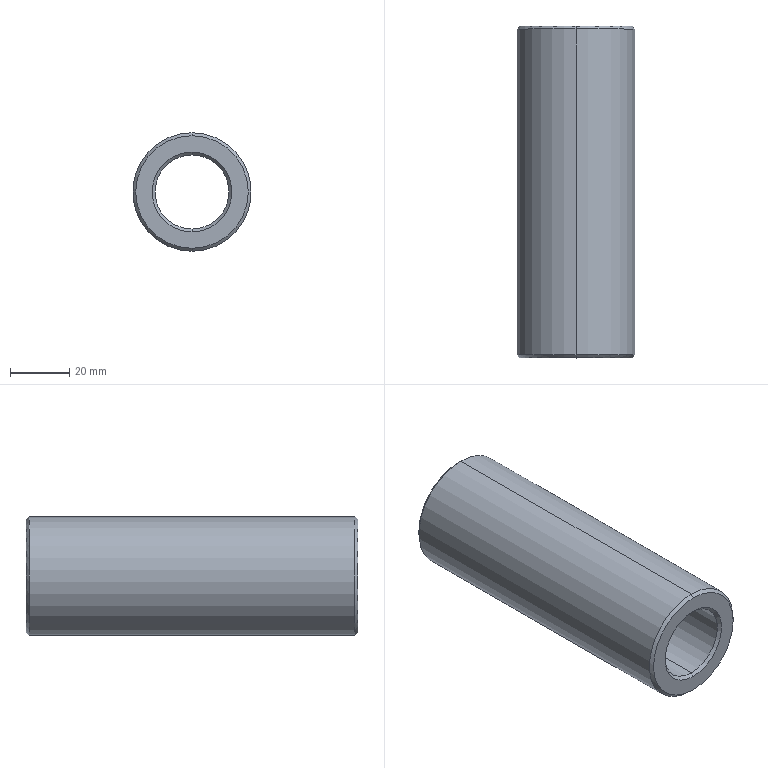Part | SolidWorks | features Chamfer 1, Extrusion 1 | 1 solid | 14 faces | box 40 x 112 x 40 mm | volume 85561 mm3 | cone 8 | cylinder 4 | plane 2 | commonest cylinder face diameters 25 x2 40 x2
STEP:
#1=CARTESIAN_POINT('',(0.,111.,-12.5));
#2=VERTEX_POINT('',#1);
#3=CARTESIAN_POINT('',(0.,111.,12.5));
#4=VERTEX_POINT('',#3);
#5=CARTESIAN_POINT('',(0.,111.,0.));
#6=DIRECTION('',(0.,1.,0.));
#7=DIRECTION('',(0.,0.,1.));
#8=AXIS2_PLACEMENT_3D('',#5,#6,#7);
#9=CIRCLE('',#8,12.5);
#10=EDGE_CURVE('',#2,#4,#9,.T.);
#11=ORIENTED_EDGE('',*,*,#10,.F.);
#12=CARTESIAN_POINT('',(0.,112.,-13.5));
#13=VERTEX_POINT('',#12);
#14=CARTESIAN_POINT('',(0.,111.,-12.5));
#15=DIRECTION('',(0.,0.7071,-0.7071));
#16=VECTOR('',#15,1000.);
#17=LINE('',#14,#16);
#18=EDGE_CURVE('',#2,#13,#17,.T.);
#19=ORIENTED_EDGE('',*,*,#18,.T.);
#20=CARTESIAN_POINT('',(0.,112.,13.5));
#21=VERTEX_POINT('',#20);
#22=CARTESIAN_POINT('',(0.,112.,0.));
#23=DIRECTION('',(0.,-1.,0.));
#24=DIRECTION('',(0.,0.,1.));
#25=AXIS2_PLACEMENT_3D('',#22,#23,#24);
#26=CIRCLE('',#25,13.5);
#27=EDGE_CURVE('',#21,#13,#26,.T.);
#28=ORIENTED_EDGE('',*,*,#27,.F.);
#29=CARTESIAN_POINT('',(0.,111.,12.5));
#30=DIRECTION('',(0.,0.7071,0.7071));
#31=VECTOR('',#30,1000.);
#32=LINE('',#29,#31);
#33=EDGE_CURVE('',#4,#21,#32,.T.);
#34=ORIENTED_EDGE('',*,*,#33,.F.);
#35=EDGE_LOOP('',(#11,#19,#28,#34));
#36=FACE_OUTER_BOUND('',#35,.T.);
#37=CARTESIAN_POINT('',(0.,111.,0.));
#38=DIRECTION('',(0.,1.,0.));
#39=DIRECTION('',(0.,0.,1.));
#40=AXIS2_PLACEMENT_3D('',#37,#38,#39);
#41=CONICAL_SURFACE('',#40,12.5,0.7854);
#42=ADVANCED_FACE('',(#36),#41,.F.);
#43=CARTESIAN_POINT('',(0.,1.,12.5));
#44=VERTEX_POINT('',#43);
#45=CARTESIAN_POINT('',(0.,1.,-12.5));
#46=VERTEX_POINT('',#45);
#47=CARTESIAN_POINT('',(0.,1.,0.));
#48=DIRECTION('',(0.,-1.,0.));
#49=DIRECTION('',(0.,0.,1.));
#50=AXIS2_PLACEMENT_3D('',#47,#48,#49);
#51=CIRCLE('',#50,12.5);
#52=EDGE_CURVE('',#44,#46,#51,.T.);
#53=ORIENTED_EDGE('',*,*,#52,.F.);
#54=CARTESIAN_POINT('',(0.,0.,13.5));
#55=VERTEX_POINT('',#54);
#56=CARTESIAN_POINT('',(0.,0.,13.5));
#57=DIRECTION('',(0.,-0.7071,0.7071));
#58=VECTOR('',#57,1000.);
#59=LINE('',#56,#58);
#60=EDGE_CURVE('',#44,#55,#59,.T.);
#61=ORIENTED_EDGE('',*,*,#60,.T.);
#62=CARTESIAN_POINT('',(0.,0.,-13.5));
#63=VERTEX_POINT('',#62);
#64=CARTESIAN_POINT('',(0.,0.,0.));
#65=DIRECTION('',(0.,1.,0.));
#66=DIRECTION('',(0.,0.,1.));
#67=AXIS2_PLACEMENT_3D('',#64,#65,#66);
#68=CIRCLE('',#67,13.5);
#69=EDGE_CURVE('',#63,#55,#68,.T.);
#70=ORIENTED_EDGE('',*,*,#69,.F.);
#71=CARTESIAN_POINT('',(0.,0.,-13.5));
#72=DIRECTION('',(0.,-0.7071,-0.7071));
#73=VECTOR('',#72,1000.);
#74=LINE('',#71,#73);
#75=EDGE_CURVE('',#46,#63,#74,.T.);
#76=ORIENTED_EDGE('',*,*,#75,.F.);
#77=EDGE_LOOP('',(#53,#61,#70,#76));
#78=FACE_OUTER_BOUND('',#77,.T.);
#79=CARTESIAN_POINT('',(0.,0.,0.));
#80=DIRECTION('',(0.,-1.,0.));
#81=DIRECTION('',(0.,0.,-1.));
#82=AXIS2_PLACEMENT_3D('',#79,#80,#81);
#83=CONICAL_SURFACE('',#82,13.5,0.7854);
#84=ADVANCED_FACE('',(#78),#83,.F.);
#85=CARTESIAN_POINT('',(0.,112.,19.));
#86=VERTEX_POINT('',#85);
#87=CARTESIAN_POINT('',(0.,112.,-19.));
#88=VERTEX_POINT('',#87);
#89=CARTESIAN_POINT('',(0.,112.,0.));
#90=DIRECTION('',(0.,1.,0.));
#91=DIRECTION('',(0.,0.,1.));
#92=AXIS2_PLACEMENT_3D('',#89,#90,#91);
#93=CIRCLE('',#92,19.);
#94=EDGE_CURVE('',#86,#88,#93,.T.);
#95=ORIENTED_EDGE('',*,*,#94,.F.);
#96=CARTESIAN_POINT('',(0.,111.,20.));
#97=VERTEX_POINT('',#96);
#98=CARTESIAN_POINT('',(0.,112.,19.));
#99=DIRECTION('',(0.,-0.7071,0.7071));
#100=VECTOR('',#99,1000.);
#101=LINE('',#98,#100);
#102=EDGE_CURVE('',#86,#97,#101,.T.);
#103=ORIENTED_EDGE('',*,*,#102,.T.);
#104=CARTESIAN_POINT('',(0.,111.,-20.));
#105=VERTEX_POINT('',#104);
#106=CARTESIAN_POINT('',(0.,111.,0.));
#107=DIRECTION('',(0.,-1.,0.));
#108=DIRECTION('',(0.,0.,1.));
#109=AXIS2_PLACEMENT_3D('',#106,#107,#108);
#110=CIRCLE('',#109,20.);
#111=EDGE_CURVE('',#105,#97,#110,.T.);
#112=ORIENTED_EDGE('',*,*,#111,.F.);
#113=CARTESIAN_POINT('',(0.,112.,-19.));
#114=DIRECTION('',(0.,-0.7071,-0.7071));
#115=VECTOR('',#114,1000.);
#116=LINE('',#113,#115);
#117=EDGE_CURVE('',#88,#105,#116,.T.);
#118=ORIENTED_EDGE('',*,*,#117,.F.);
#119=EDGE_LOOP('',(#95,#103,#112,#118));
#120=FACE_OUTER_BOUND('',#119,.T.);
#121=CARTESIAN_POINT('',(0.,112.,0.));
#122=DIRECTION('',(0.,-1.,0.));
#123=DIRECTION('',(0.,0.,-1.));
#124=AXIS2_PLACEMENT_3D('',#121,#122,#123);
#125=CONICAL_SURFACE('',#124,19.,0.7854);
#126=ADVANCED_FACE('',(#120),#125,.T.);
#127=CARTESIAN_POINT('',(0.,0.,-19.));
#128=VERTEX_POINT('',#127);
#129=CARTESIAN_POINT('',(0.,0.,19.));
#130=VERTEX_POINT('',#129);
#131=CARTESIAN_POINT('',(0.,0.,0.));
#132=DIRECTION('',(0.,-1.,0.));
#133=DIRECTION('',(0.,0.,1.));
#134=AXIS2_PLACEMENT_3D('',#131,#132,#133);
#135=CIRCLE('',#134,19.);
#136=EDGE_CURVE('',#128,#130,#135,.T.);
#137=ORIENTED_EDGE('',*,*,#136,.F.);
#138=CARTESIAN_POINT('',(0.,1.,-20.));
#139=VERTEX_POINT('',#138);
#140=CARTESIAN_POINT('',(0.,1.,-20.));
#141=DIRECTION('',(0.,0.7071,-0.7071));
#142=VECTOR('',#141,1000.);
#143=LINE('',#140,#142);
#144=EDGE_CURVE('',#128,#139,#143,.T.);
#145=ORIENTED_EDGE('',*,*,#144,.T.);
#146=CARTESIAN_POINT('',(0.,1.,20.));
#147=VERTEX_POINT('',#146);
#148=CARTESIAN_POINT('',(0.,1.,0.));
#149=DIRECTION('',(0.,1.,0.));
#150=DIRECTION('',(0.,0.,1.));
#151=AXIS2_PLACEMENT_3D('',#148,#149,#150);
#152=CIRCLE('',#151,20.);
#153=EDGE_CURVE('',#147,#139,#152,.T.);
#154=ORIENTED_EDGE('',*,*,#153,.F.);
#155=CARTESIAN_POINT('',(0.,1.,20.));
#156=DIRECTION('',(0.,0.7071,0.7071));
#157=VECTOR('',#156,1000.);
#158=LINE('',#155,#157);
#159=EDGE_CURVE('',#130,#147,#158,.T.);
#160=ORIENTED_EDGE('',*,*,#159,.F.);
#161=EDGE_LOOP('',(#137,#145,#154,#160));
#162=FACE_OUTER_BOUND('',#161,.T.);
#163=CARTESIAN_POINT('',(0.,1.,0.));
#164=DIRECTION('',(0.,1.,0.));
#165=DIRECTION('',(0.,0.,1.));
#166=AXIS2_PLACEMENT_3D('',#163,#164,#165);
#167=CONICAL_SURFACE('',#166,20.,0.7854);
#168=ADVANCED_FACE('',(#162),#167,.T.);
#169=ORIENTED_EDGE('',*,*,#10,.T.);
#170=CARTESIAN_POINT('',(0.,112.,12.5));
#171=DIRECTION('',(0.,-1.,0.));
#172=VECTOR('',#171,1000.);
#173=LINE('',#170,#172);
#174=EDGE_CURVE('',#4,#44,#173,.T.);
#175=ORIENTED_EDGE('',*,*,#174,.T.);
#176=ORIENTED_EDGE('',*,*,#52,.T.);
#177=CARTESIAN_POINT('',(0.,112.,-12.5));
#178=DIRECTION('',(0.,-1.,0.));
#179=VECTOR('',#178,1000.);
#180=LINE('',#177,#179);
#181=EDGE_CURVE('',#2,#46,#180,.T.);
#182=ORIENTED_EDGE('',*,*,#181,.F.);
#183=EDGE_LOOP('',(#169,#175,#176,#182));
#184=FACE_OUTER_BOUND('',#183,.T.);
#185=CARTESIAN_POINT('',(0.,112.,0.));
#186=DIRECTION('',(0.,-1.,0.));
#187=DIRECTION('',(0.,0.,-1.));
#188=AXIS2_PLACEMENT_3D('',#185,#186,#187);
#189=CYLINDRICAL_SURFACE('',#188,12.5);
#190=ADVANCED_FACE('',(#184),#189,.F.);
#191=ORIENTED_EDGE('',*,*,#111,.T.);
#192=CARTESIAN_POINT('',(0.,112.,20.));
#193=DIRECTION('',(0.,-1.,0.));
#194=VECTOR('',#193,1000.);
#195=LINE('',#192,#194);
#196=EDGE_CURVE('',#97,#147,#195,.T.);
#197=ORIENTED_EDGE('',*,*,#196,.T.);
#198=ORIENTED_EDGE('',*,*,#153,.T.);
#199=CARTESIAN_POINT('',(0.,112.,-20.));
#200=DIRECTION('',(0.,-1.,0.));
#201=VECTOR('',#200,1000.);
#202=LINE('',#199,#201);
#203=EDGE_CURVE('',#105,#139,#202,.T.);
#204=ORIENTED_EDGE('',*,*,#203,.F.);
#205=EDGE_LOOP('',(#191,#197,#198,#204));
#206=FACE_OUTER_BOUND('',#205,.T.);
#207=CARTESIAN_POINT('',(0.,112.,0.));
#208=DIRECTION('',(0.,-1.,0.));
#209=DIRECTION('',(0.,0.,-1.));
#210=AXIS2_PLACEMENT_3D('',#207,#208,#209);
#211=CYLINDRICAL_SURFACE('',#210,20.);
#212=ADVANCED_FACE('',(#206),#211,.T.);
#213=CARTESIAN_POINT('',(0.,112.,0.));
#214=DIRECTION('',(0.,1.,0.));
#215=DIRECTION('',(0.,0.,1.));
#216=AXIS2_PLACEMENT_3D('',#213,#214,#215);
#217=CIRCLE('',#216,19.);
#218=EDGE_CURVE('',#88,#86,#217,.T.);
#219=ORIENTED_EDGE('',*,*,#218,.T.);
#220=ORIENTED_EDGE('',*,*,#94,.T.);
#221=EDGE_LOOP('',(#219,#220));
#222=FACE_OUTER_BOUND('',#221,.T.);
#223=ORIENTED_EDGE('',*,*,#27,.T.);
#224=CARTESIAN_POINT('',(0.,112.,0.));
#225=DIRECTION('',(0.,-1.,0.));
#226=DIRECTION('',(0.,0.,1.));
#227=AXIS2_PLACEMENT_3D('',#224,#225,#226);
#228=CIRCLE('',#227,13.5);
#229=EDGE_CURVE('',#13,#21,#228,.T.);
#230=ORIENTED_EDGE('',*,*,#229,.T.);
#231=EDGE_LOOP('',(#223,#230));
#232=FACE_BOUND('',#231,.T.);
#233=CARTESIAN_POINT('',(0.,112.,0.));
#234=DIRECTION('',(0.,1.,0.));
#235=DIRECTION('',(0.,0.,1.));
#236=AXIS2_PLACEMENT_3D('',#233,#234,#235);
#237=PLANE('',#236);
#238=ADVANCED_FACE('',(#222,#232),#237,.T.);
#239=CARTESIAN_POINT('',(0.,0.,0.));
#240=DIRECTION('',(0.,-1.,0.));
#241=DIRECTION('',(0.,0.,1.));
#242=AXIS2_PLACEMENT_3D('',#239,#240,#241);
#243=CIRCLE('',#242,19.);
#244=EDGE_CURVE('',#130,#128,#243,.T.);
#245=ORIENTED_EDGE('',*,*,#244,.T.);
#246=ORIENTED_EDGE('',*,*,#136,.T.);
#247=EDGE_LOOP('',(#245,#246));
#248=FACE_OUTER_BOUND('',#247,.T.);
#249=ORIENTED_EDGE('',*,*,#69,.T.);
#250=CARTESIAN_POINT('',(0.,0.,0.));
#251=DIRECTION('',(0.,1.,0.));
#252=DIRECTION('',(0.,0.,1.));
#253=AXIS2_PLACEMENT_3D('',#250,#251,#252);
#254=CIRCLE('',#253,13.5);
#255=EDGE_CURVE('',#55,#63,#254,.T.);
#256=ORIENTED_EDGE('',*,*,#255,.T.);
#257=EDGE_LOOP('',(#249,#256));
#258=FACE_BOUND('',#257,.T.);
#259=CARTESIAN_POINT('',(0.,0.,0.));
#260=DIRECTION('',(0.,1.,0.));
#261=DIRECTION('',(0.,0.,1.));
#262=AXIS2_PLACEMENT_3D('',#259,#260,#261);
#263=PLANE('',#262);
#264=ADVANCED_FACE('',(#248,#258),#263,.F.);
#265=ORIENTED_EDGE('',*,*,#196,.F.);
#266=CARTESIAN_POINT('',(0.,111.,0.));
#267=DIRECTION('',(0.,-1.,0.));
#268=DIRECTION('',(0.,0.,1.));
#269=AXIS2_PLACEMENT_3D('',#266,#267,#268);
#270=CIRCLE('',#269,20.);
#271=EDGE_CURVE('',#97,#105,#270,.T.);
#272=ORIENTED_EDGE('',*,*,#271,.T.);
#273=ORIENTED_EDGE('',*,*,#203,.T.);
#274=CARTESIAN_POINT('',(0.,1.,0.));
#275=DIRECTION('',(0.,1.,0.));
#276=DIRECTION('',(0.,0.,1.));
#277=AXIS2_PLACEMENT_3D('',#274,#275,#276);
#278=CIRCLE('',#277,20.);
#279=EDGE_CURVE('',#139,#147,#278,.T.);
#280=ORIENTED_EDGE('',*,*,#279,.T.);
#281=EDGE_LOOP('',(#265,#272,#273,#280));
#282=FACE_OUTER_BOUND('',#281,.T.);
#283=CARTESIAN_POINT('',(0.,112.,0.));
#284=DIRECTION('',(0.,-1.,0.));
#285=DIRECTION('',(0.,0.,-1.));
#286=AXIS2_PLACEMENT_3D('',#283,#284,#285);
#287=CYLINDRICAL_SURFACE('',#286,20.);
#288=ADVANCED_FACE('',(#282),#287,.T.);
#289=ORIENTED_EDGE('',*,*,#174,.F.);
#290=CARTESIAN_POINT('',(0.,111.,0.));
#291=DIRECTION('',(0.,1.,0.));
#292=DIRECTION('',(0.,0.,1.));
#293=AXIS2_PLACEMENT_3D('',#290,#291,#292);
#294=CIRCLE('',#293,12.5);
#295=EDGE_CURVE('',#4,#2,#294,.T.);
#296=ORIENTED_EDGE('',*,*,#295,.T.);
#297=ORIENTED_EDGE('',*,*,#181,.T.);
#298=CARTESIAN_POINT('',(0.,1.,0.));
#299=DIRECTION('',(0.,-1.,0.));
#300=DIRECTION('',(0.,0.,1.));
#301=AXIS2_PLACEMENT_3D('',#298,#299,#300);
#302=CIRCLE('',#301,12.5);
#303=EDGE_CURVE('',#46,#44,#302,.T.);
#304=ORIENTED_EDGE('',*,*,#303,.T.);
#305=EDGE_LOOP('',(#289,#296,#297,#304));
#306=FACE_OUTER_BOUND('',#305,.T.);
#307=CARTESIAN_POINT('',(0.,112.,0.));
#308=DIRECTION('',(0.,-1.,0.));
#309=DIRECTION('',(0.,0.,-1.));
#310=AXIS2_PLACEMENT_3D('',#307,#308,#309);
#311=CYLINDRICAL_SURFACE('',#310,12.5);
#312=ADVANCED_FACE('',(#306),#311,.F.);
#313=ORIENTED_EDGE('',*,*,#144,.F.);
#314=ORIENTED_EDGE('',*,*,#244,.F.);
#315=ORIENTED_EDGE('',*,*,#159,.T.);
#316=ORIENTED_EDGE('',*,*,#279,.F.);
#317=EDGE_LOOP('',(#313,#314,#315,#316));
#318=FACE_OUTER_BOUND('',#317,.T.);
#319=CARTESIAN_POINT('',(0.,1.,0.));
#320=DIRECTION('',(0.,1.,0.));
#321=DIRECTION('',(0.,0.,1.));
#322=AXIS2_PLACEMENT_3D('',#319,#320,#321);
#323=CONICAL_SURFACE('',#322,20.,0.7854);
#324=ADVANCED_FACE('',(#318),#323,.T.);
#325=ORIENTED_EDGE('',*,*,#102,.F.);
#326=ORIENTED_EDGE('',*,*,#218,.F.);
#327=ORIENTED_EDGE('',*,*,#117,.T.);
#328=ORIENTED_EDGE('',*,*,#271,.F.);
#329=EDGE_LOOP('',(#325,#326,#327,#328));
#330=FACE_OUTER_BOUND('',#329,.T.);
#331=CARTESIAN_POINT('',(0.,112.,0.));
#332=DIRECTION('',(0.,-1.,0.));
#333=DIRECTION('',(0.,0.,-1.));
#334=AXIS2_PLACEMENT_3D('',#331,#332,#333);
#335=CONICAL_SURFACE('',#334,19.,0.7854);
#336=ADVANCED_FACE('',(#330),#335,.T.);
#337=ORIENTED_EDGE('',*,*,#60,.F.);
#338=ORIENTED_EDGE('',*,*,#303,.F.);
#339=ORIENTED_EDGE('',*,*,#75,.T.);
#340=ORIENTED_EDGE('',*,*,#255,.F.);
#341=EDGE_LOOP('',(#337,#338,#339,#340));
#342=FACE_OUTER_BOUND('',#341,.T.);
#343=CARTESIAN_POINT('',(0.,0.,0.));
#344=DIRECTION('',(0.,-1.,0.));
#345=DIRECTION('',(0.,0.,-1.));
#346=AXIS2_PLACEMENT_3D('',#343,#344,#345);
#347=CONICAL_SURFACE('',#346,13.5,0.7854);
#348=ADVANCED_FACE('',(#342),#347,.F.);
#349=ORIENTED_EDGE('',*,*,#18,.F.);
#350=ORIENTED_EDGE('',*,*,#295,.F.);
#351=ORIENTED_EDGE('',*,*,#33,.T.);
#352=ORIENTED_EDGE('',*,*,#229,.F.);
#353=EDGE_LOOP('',(#349,#350,#351,#352));
#354=FACE_OUTER_BOUND('',#353,.T.);
#355=CARTESIAN_POINT('',(0.,111.,0.));
#356=DIRECTION('',(0.,1.,0.));
#357=DIRECTION('',(0.,0.,1.));
#358=AXIS2_PLACEMENT_3D('',#355,#356,#357);
#359=CONICAL_SURFACE('',#358,12.5,0.7854);
#360=ADVANCED_FACE('',(#354),#359,.F.);
#361=CLOSED_SHELL('',(#42,#84,#126,#168,#190,#212,#238,#264,#288,#312,#324,#336,#348,#360));
#362=MANIFOLD_SOLID_BREP('',#361);
#363=CARTESIAN_POINT('',(0.,0.,0.));
#364=DIRECTION('',(0.,0.,1.));
#365=DIRECTION('',(1.,0.,0.));
#366=AXIS2_PLACEMENT_3D('',#363,#364,#365);
#367=(LENGTH_UNIT()NAMED_UNIT(*)SI_UNIT(.MILLI.,.METRE.));
#368=UNCERTAINTY_MEASURE_WITH_UNIT(LENGTH_MEASURE(0.00001),#367,'','');
#369=(NAMED_UNIT(*)PLANE_ANGLE_UNIT()SI_UNIT($,.RADIAN.));
#370=(NAMED_UNIT(*)SI_UNIT($,.STERADIAN.)SOLID_ANGLE_UNIT());
#371=(GEOMETRIC_REPRESENTATION_CONTEXT(3)GLOBAL_UNCERTAINTY_ASSIGNED_CONTEXT((#368))GLOBAL_UNIT_ASSIGNED_CONTEXT((#367,#369,#370))REPRESENTATION_CONTEXT('',''));
#372=ADVANCED_BREP_SHAPE_REPRESENTATION('',(#362,#366),#371);